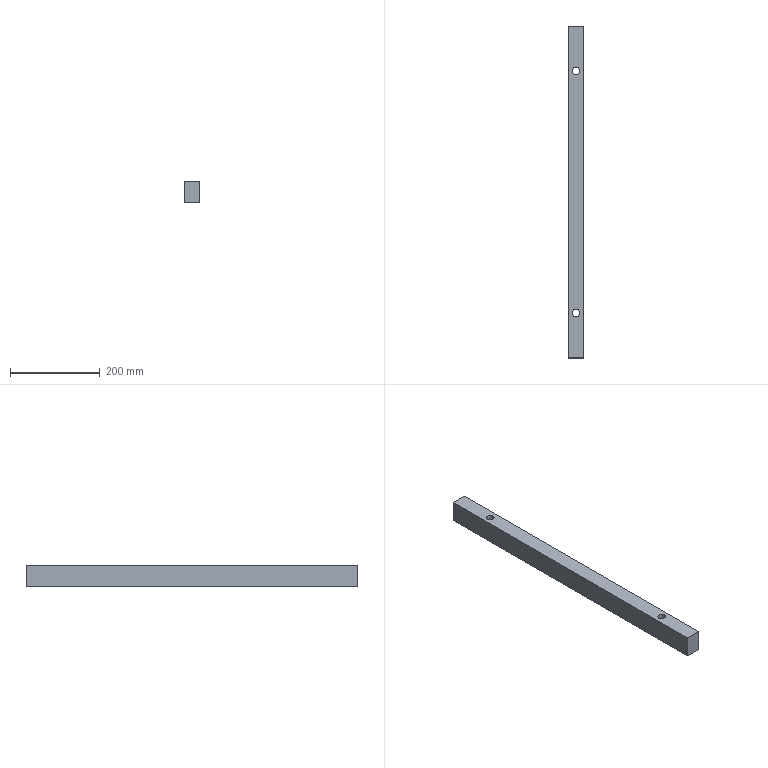Part | NX | features solid 2 | 1 solid | 8 faces | box 35 x 740 x 49 mm | volume 1246856 mm3 | plane 6 | cylinder 2 | commonest cylinder face diameters 17 x2
STEP:
#1=CARTESIAN_POINT('',(255.5,-370.,202.));
#2=VERTEX_POINT('',#1);
#3=CARTESIAN_POINT('',(255.5,370.,202.));
#4=VERTEX_POINT('',#3);
#5=CARTESIAN_POINT('',(255.5,0.,202.));
#6=DIRECTION('',(0.,1.,0.));
#7=VECTOR('',#6,1000.);
#8=LINE('',#5,#7);
#9=EDGE_CURVE('',#2,#4,#8,.T.);
#10=ORIENTED_EDGE('',*,*,#9,.T.);
#11=CARTESIAN_POINT('',(255.5,370.,153.));
#12=VERTEX_POINT('',#11);
#13=CARTESIAN_POINT('',(255.5,370.,148.));
#14=DIRECTION('',(0.,0.,1.));
#15=VECTOR('',#14,1000.);
#16=LINE('',#13,#15);
#17=EDGE_CURVE('',#12,#4,#16,.T.);
#18=ORIENTED_EDGE('',*,*,#17,.F.);
#19=CARTESIAN_POINT('',(255.5,-370.,153.));
#20=VERTEX_POINT('',#19);
#21=CARTESIAN_POINT('',(255.5,0.,153.));
#22=DIRECTION('',(0.,-1.,0.));
#23=VECTOR('',#22,1000.);
#24=LINE('',#21,#23);
#25=EDGE_CURVE('',#12,#20,#24,.T.);
#26=ORIENTED_EDGE('',*,*,#25,.T.);
#27=CARTESIAN_POINT('',(255.5,-370.,148.));
#28=DIRECTION('',(0.,0.,1.));
#29=VECTOR('',#28,1000.);
#30=LINE('',#27,#29);
#31=EDGE_CURVE('',#20,#2,#30,.T.);
#32=ORIENTED_EDGE('',*,*,#31,.T.);
#33=EDGE_LOOP('',(#10,#18,#26,#32));
#34=FACE_BOUND('',#33,.T.);
#35=CARTESIAN_POINT('',(255.5,0.,148.));
#36=DIRECTION('',(-1.,0.,0.));
#37=DIRECTION('',(0.,0.,1.));
#38=AXIS2_PLACEMENT_3D('',#35,#36,#37);
#39=PLANE('',#38);
#40=ADVANCED_FACE('',(#34),#39,.T.);
#41=CARTESIAN_POINT('',(290.5,-370.,153.));
#42=VERTEX_POINT('',#41);
#43=CARTESIAN_POINT('',(290.5,370.,153.));
#44=VERTEX_POINT('',#43);
#45=CARTESIAN_POINT('',(290.5,0.,153.));
#46=DIRECTION('',(0.,1.,0.));
#47=VECTOR('',#46,1000.);
#48=LINE('',#45,#47);
#49=EDGE_CURVE('',#42,#44,#48,.T.);
#50=ORIENTED_EDGE('',*,*,#49,.T.);
#51=CARTESIAN_POINT('',(290.5,370.,202.));
#52=VERTEX_POINT('',#51);
#53=CARTESIAN_POINT('',(290.5,370.,148.));
#54=DIRECTION('',(0.,0.,1.));
#55=VECTOR('',#54,1000.);
#56=LINE('',#53,#55);
#57=EDGE_CURVE('',#44,#52,#56,.T.);
#58=ORIENTED_EDGE('',*,*,#57,.T.);
#59=CARTESIAN_POINT('',(290.5,-370.,202.));
#60=VERTEX_POINT('',#59);
#61=CARTESIAN_POINT('',(290.5,0.,202.));
#62=DIRECTION('',(0.,-1.,0.));
#63=VECTOR('',#62,1000.);
#64=LINE('',#61,#63);
#65=EDGE_CURVE('',#52,#60,#64,.T.);
#66=ORIENTED_EDGE('',*,*,#65,.T.);
#67=CARTESIAN_POINT('',(290.5,-370.,148.));
#68=DIRECTION('',(0.,0.,1.));
#69=VECTOR('',#68,1000.);
#70=LINE('',#67,#69);
#71=EDGE_CURVE('',#42,#60,#70,.T.);
#72=ORIENTED_EDGE('',*,*,#71,.F.);
#73=EDGE_LOOP('',(#50,#58,#66,#72));
#74=FACE_BOUND('',#73,.T.);
#75=CARTESIAN_POINT('',(290.5,0.,148.));
#76=DIRECTION('',(1.,0.,0.));
#77=DIRECTION('',(0.,0.,-1.));
#78=AXIS2_PLACEMENT_3D('',#75,#76,#77);
#79=PLANE('',#78);
#80=ADVANCED_FACE('',(#74),#79,.T.);
#81=ORIENTED_EDGE('',*,*,#65,.F.);
#82=CARTESIAN_POINT('',(273.,370.,202.));
#83=DIRECTION('',(1.,0.,0.));
#84=VECTOR('',#83,1000.);
#85=LINE('',#82,#84);
#86=EDGE_CURVE('',#4,#52,#85,.T.);
#87=ORIENTED_EDGE('',*,*,#86,.F.);
#88=ORIENTED_EDGE('',*,*,#9,.F.);
#89=CARTESIAN_POINT('',(273.,-370.,202.));
#90=DIRECTION('',(-1.,0.,0.));
#91=VECTOR('',#90,1000.);
#92=LINE('',#89,#91);
#93=EDGE_CURVE('',#60,#2,#92,.T.);
#94=ORIENTED_EDGE('',*,*,#93,.F.);
#95=EDGE_LOOP('',(#81,#87,#88,#94));
#96=FACE_BOUND('',#95,.T.);
#97=CARTESIAN_POINT('',(264.5,-270.,202.));
#98=VERTEX_POINT('',#97);
#99=CARTESIAN_POINT('',(273.,-270.,202.));
#100=DIRECTION('',(0.,0.,1.));
#101=DIRECTION('',(-1.,0.,0.));
#102=AXIS2_PLACEMENT_3D('',#99,#100,#101);
#103=CIRCLE('',#102,8.5);
#104=EDGE_CURVE('',#98,#98,#103,.F.);
#105=ORIENTED_EDGE('',*,*,#104,.T.);
#106=EDGE_LOOP('',(#105));
#107=FACE_BOUND('',#106,.T.);
#108=CARTESIAN_POINT('',(264.5,270.,202.));
#109=VERTEX_POINT('',#108);
#110=CARTESIAN_POINT('',(273.,270.,202.));
#111=DIRECTION('',(0.,0.,-1.));
#112=DIRECTION('',(-1.,0.,0.));
#113=AXIS2_PLACEMENT_3D('',#110,#111,#112);
#114=CIRCLE('',#113,8.5);
#115=EDGE_CURVE('',#109,#109,#114,.T.);
#116=ORIENTED_EDGE('',*,*,#115,.T.);
#117=EDGE_LOOP('',(#116));
#118=FACE_BOUND('',#117,.T.);
#119=CARTESIAN_POINT('',(273.,0.,202.));
#120=DIRECTION('',(0.,0.,1.));
#121=DIRECTION('',(1.,0.,0.));
#122=AXIS2_PLACEMENT_3D('',#119,#120,#121);
#123=PLANE('',#122);
#124=ADVANCED_FACE('',(#96,#107,#118),#123,.T.);
#125=ORIENTED_EDGE('',*,*,#25,.F.);
#126=CARTESIAN_POINT('',(273.,370.,153.));
#127=DIRECTION('',(-1.,0.,0.));
#128=VECTOR('',#127,1000.);
#129=LINE('',#126,#128);
#130=EDGE_CURVE('',#44,#12,#129,.T.);
#131=ORIENTED_EDGE('',*,*,#130,.F.);
#132=ORIENTED_EDGE('',*,*,#49,.F.);
#133=CARTESIAN_POINT('',(273.,-370.,153.));
#134=DIRECTION('',(1.,0.,0.));
#135=VECTOR('',#134,1000.);
#136=LINE('',#133,#135);
#137=EDGE_CURVE('',#20,#42,#136,.T.);
#138=ORIENTED_EDGE('',*,*,#137,.F.);
#139=EDGE_LOOP('',(#125,#131,#132,#138));
#140=FACE_BOUND('',#139,.T.);
#141=CARTESIAN_POINT('',(264.5,-270.,153.));
#142=VERTEX_POINT('',#141);
#143=CARTESIAN_POINT('',(273.,-270.,153.));
#144=DIRECTION('',(0.,0.,-1.));
#145=DIRECTION('',(-1.,0.,0.));
#146=AXIS2_PLACEMENT_3D('',#143,#144,#145);
#147=CIRCLE('',#146,8.5);
#148=EDGE_CURVE('',#142,#142,#147,.F.);
#149=ORIENTED_EDGE('',*,*,#148,.T.);
#150=EDGE_LOOP('',(#149));
#151=FACE_BOUND('',#150,.T.);
#152=CARTESIAN_POINT('',(264.5,270.,153.));
#153=VERTEX_POINT('',#152);
#154=CARTESIAN_POINT('',(273.,270.,153.));
#155=DIRECTION('',(0.,0.,-1.));
#156=DIRECTION('',(-1.,0.,0.));
#157=AXIS2_PLACEMENT_3D('',#154,#155,#156);
#158=CIRCLE('',#157,8.5);
#159=EDGE_CURVE('',#153,#153,#158,.F.);
#160=ORIENTED_EDGE('',*,*,#159,.T.);
#161=EDGE_LOOP('',(#160));
#162=FACE_BOUND('',#161,.T.);
#163=CARTESIAN_POINT('',(785.5,0.,153.));
#164=DIRECTION('',(0.,0.,-1.));
#165=DIRECTION('',(-1.,0.,0.));
#166=AXIS2_PLACEMENT_3D('',#163,#164,#165);
#167=PLANE('',#166);
#168=ADVANCED_FACE('',(#140,#151,#162),#167,.T.);
#169=ORIENTED_EDGE('',*,*,#104,.F.);
#170=EDGE_LOOP('',(#169));
#171=FACE_BOUND('',#170,.T.);
#172=ORIENTED_EDGE('',*,*,#148,.F.);
#173=EDGE_LOOP('',(#172));
#174=FACE_BOUND('',#173,.T.);
#175=CARTESIAN_POINT('',(273.,-270.,202.));
#176=DIRECTION('',(0.,0.,-1.));
#177=DIRECTION('',(-1.,0.,0.));
#178=AXIS2_PLACEMENT_3D('',#175,#176,#177);
#179=CYLINDRICAL_SURFACE('',#178,8.5);
#180=ADVANCED_FACE('',(#171,#174),#179,.F.);
#181=ORIENTED_EDGE('',*,*,#31,.F.);
#182=ORIENTED_EDGE('',*,*,#137,.T.);
#183=ORIENTED_EDGE('',*,*,#71,.T.);
#184=ORIENTED_EDGE('',*,*,#93,.T.);
#185=EDGE_LOOP('',(#181,#182,#183,#184));
#186=FACE_BOUND('',#185,.T.);
#187=CARTESIAN_POINT('',(273.,-370.,148.));
#188=DIRECTION('',(0.,-1.,0.));
#189=DIRECTION('',(0.,0.,-1.));
#190=AXIS2_PLACEMENT_3D('',#187,#188,#189);
#191=PLANE('',#190);
#192=ADVANCED_FACE('',(#186),#191,.T.);
#193=ORIENTED_EDGE('',*,*,#115,.F.);
#194=EDGE_LOOP('',(#193));
#195=FACE_BOUND('',#194,.T.);
#196=ORIENTED_EDGE('',*,*,#159,.F.);
#197=EDGE_LOOP('',(#196));
#198=FACE_BOUND('',#197,.T.);
#199=CARTESIAN_POINT('',(273.,270.,202.));
#200=DIRECTION('',(0.,0.,-1.));
#201=DIRECTION('',(-1.,0.,0.));
#202=AXIS2_PLACEMENT_3D('',#199,#200,#201);
#203=CYLINDRICAL_SURFACE('',#202,8.5);
#204=ADVANCED_FACE('',(#195,#198),#203,.F.);
#205=ORIENTED_EDGE('',*,*,#57,.F.);
#206=ORIENTED_EDGE('',*,*,#130,.T.);
#207=ORIENTED_EDGE('',*,*,#17,.T.);
#208=ORIENTED_EDGE('',*,*,#86,.T.);
#209=EDGE_LOOP('',(#205,#206,#207,#208));
#210=FACE_BOUND('',#209,.T.);
#211=CARTESIAN_POINT('',(273.,370.,148.));
#212=DIRECTION('',(0.,1.,0.));
#213=DIRECTION('',(0.,0.,1.));
#214=AXIS2_PLACEMENT_3D('',#211,#212,#213);
#215=PLANE('',#214);
#216=ADVANCED_FACE('',(#210),#215,.T.);
#217=CLOSED_SHELL('',(#40,#80,#124,#168,#180,#192,#204,#216));
#218=MANIFOLD_SOLID_BREP('',#217);
#219=(LENGTH_UNIT()NAMED_UNIT(*)SI_UNIT(.MILLI.,.METRE.));
#220=UNCERTAINTY_MEASURE_WITH_UNIT(LENGTH_MEASURE(0.00001),#219,'','');
#221=(NAMED_UNIT(*)PLANE_ANGLE_UNIT()SI_UNIT($,.RADIAN.));
#222=(NAMED_UNIT(*)SI_UNIT($,.STERADIAN.)SOLID_ANGLE_UNIT());
#223=(GEOMETRIC_REPRESENTATION_CONTEXT(3)GLOBAL_UNCERTAINTY_ASSIGNED_CONTEXT((#220))GLOBAL_UNIT_ASSIGNED_CONTEXT((#219,#221,#222))REPRESENTATION_CONTEXT('',''));
#224=ADVANCED_BREP_SHAPE_REPRESENTATION('',(#218),#223);